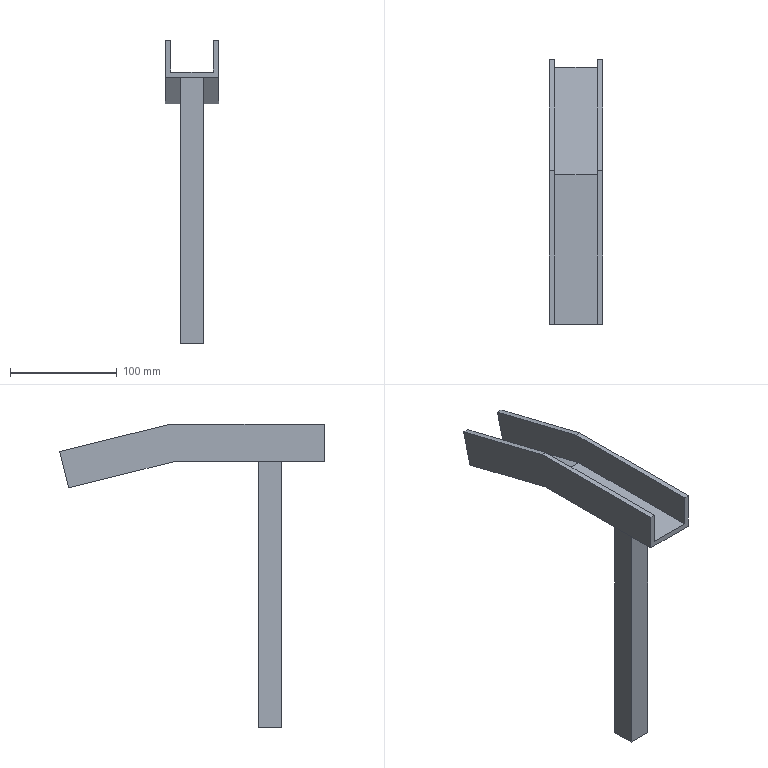Part | NX | features solid 2 | 1 solid | 24 faces | box 50 x 248.417 x 285 mm | volume 175280 mm3 | plane 24
STEP:
#1=CARTESIAN_POINT('',(228.742,734.,15.));
#2=VERTEX_POINT('',#1);
#3=CARTESIAN_POINT('',(228.742,874.61,15.));
#4=VERTEX_POINT('',#3);
#5=CARTESIAN_POINT('',(228.742,829.805,15.));
#6=DIRECTION('',(0.,1.,0.));
#7=VECTOR('',#6,1000.);
#8=LINE('',#5,#7);
#9=EDGE_CURVE('',#2,#4,#8,.T.);
#10=ORIENTED_EDGE('',*,*,#9,.T.);
#11=CARTESIAN_POINT('',(228.742,975.202,-9.923));
#12=VERTEX_POINT('',#11);
#13=CARTESIAN_POINT('',(228.742,924.906,2.538));
#14=DIRECTION('',(0.,0.9707,-0.2405));
#15=VECTOR('',#14,1000.);
#16=LINE('',#13,#15);
#17=EDGE_CURVE('',#4,#12,#16,.T.);
#18=ORIENTED_EDGE('',*,*,#17,.T.);
#19=CARTESIAN_POINT('',(228.742,982.417,19.196));
#20=VERTEX_POINT('',#19);
#21=CARTESIAN_POINT('',(228.742,978.81,4.637));
#22=DIRECTION('',(0.,0.2405,0.9707));
#23=VECTOR('',#22,1000.);
#24=LINE('',#21,#23);
#25=EDGE_CURVE('',#12,#20,#24,.T.);
#26=ORIENTED_EDGE('',*,*,#25,.T.);
#27=CARTESIAN_POINT('',(228.742,878.271,45.));
#28=VERTEX_POINT('',#27);
#29=CARTESIAN_POINT('',(228.742,930.344,32.098));
#30=DIRECTION('',(0.,0.9707,-0.2405));
#31=VECTOR('',#30,1000.);
#32=LINE('',#29,#31);
#33=EDGE_CURVE('',#28,#20,#32,.T.);
#34=ORIENTED_EDGE('',*,*,#33,.F.);
#35=CARTESIAN_POINT('',(228.742,734.,45.));
#36=VERTEX_POINT('',#35);
#37=CARTESIAN_POINT('',(228.742,831.636,45.));
#38=DIRECTION('',(0.,1.,0.));
#39=VECTOR('',#38,1000.);
#40=LINE('',#37,#39);
#41=EDGE_CURVE('',#36,#28,#40,.T.);
#42=ORIENTED_EDGE('',*,*,#41,.F.);
#43=CARTESIAN_POINT('',(228.742,734.,10.));
#44=DIRECTION('',(0.,0.,1.));
#45=VECTOR('',#44,1000.);
#46=LINE('',#43,#45);
#47=EDGE_CURVE('',#2,#36,#46,.T.);
#48=ORIENTED_EDGE('',*,*,#47,.F.);
#49=EDGE_LOOP('',(#10,#18,#26,#34,#42,#48));
#50=FACE_BOUND('',#49,.T.);
#51=CARTESIAN_POINT('',(228.742,831.636,45.));
#52=DIRECTION('',(1.,0.,0.));
#53=DIRECTION('',(0.,0.,1.));
#54=AXIS2_PLACEMENT_3D('',#51,#52,#53);
#55=PLANE('',#54);
#56=ADVANCED_FACE('',(#50),#55,.T.);
#57=CARTESIAN_POINT('',(268.742,734.,15.));
#58=VERTEX_POINT('',#57);
#59=CARTESIAN_POINT('',(268.742,874.61,15.));
#60=VERTEX_POINT('',#59);
#61=CARTESIAN_POINT('',(268.742,829.805,15.));
#62=DIRECTION('',(0.,1.,0.));
#63=VECTOR('',#62,1000.);
#64=LINE('',#61,#63);
#65=EDGE_CURVE('',#58,#60,#64,.T.);
#66=ORIENTED_EDGE('',*,*,#65,.T.);
#67=CARTESIAN_POINT('',(248.742,874.61,15.));
#68=DIRECTION('',(-1.,0.,0.));
#69=VECTOR('',#68,1000.);
#70=LINE('',#67,#69);
#71=EDGE_CURVE('',#60,#4,#70,.T.);
#72=ORIENTED_EDGE('',*,*,#71,.T.);
#73=ORIENTED_EDGE('',*,*,#9,.F.);
#74=CARTESIAN_POINT('',(137.742,734.,15.));
#75=DIRECTION('',(-1.,0.,0.));
#76=VECTOR('',#75,1000.);
#77=LINE('',#74,#76);
#78=EDGE_CURVE('',#58,#2,#77,.T.);
#79=ORIENTED_EDGE('',*,*,#78,.F.);
#80=EDGE_LOOP('',(#66,#72,#73,#79));
#81=FACE_BOUND('',#80,.T.);
#82=CARTESIAN_POINT('',(228.742,829.805,15.));
#83=DIRECTION('',(0.,0.,1.));
#84=DIRECTION('',(0.,1.,0.));
#85=AXIS2_PLACEMENT_3D('',#82,#83,#84);
#86=PLANE('',#85);
#87=ADVANCED_FACE('',(#81),#86,.T.);
#88=CARTESIAN_POINT('',(268.742,734.,45.));
#89=VERTEX_POINT('',#88);
#90=CARTESIAN_POINT('',(268.742,878.271,45.));
#91=VERTEX_POINT('',#90);
#92=CARTESIAN_POINT('',(268.742,831.636,45.));
#93=DIRECTION('',(0.,1.,0.));
#94=VECTOR('',#93,1000.);
#95=LINE('',#92,#94);
#96=EDGE_CURVE('',#89,#91,#95,.T.);
#97=ORIENTED_EDGE('',*,*,#96,.T.);
#98=CARTESIAN_POINT('',(268.742,982.417,19.196));
#99=VERTEX_POINT('',#98);
#100=CARTESIAN_POINT('',(268.742,930.344,32.098));
#101=DIRECTION('',(0.,0.9707,-0.2405));
#102=VECTOR('',#101,1000.);
#103=LINE('',#100,#102);
#104=EDGE_CURVE('',#91,#99,#103,.T.);
#105=ORIENTED_EDGE('',*,*,#104,.T.);
#106=CARTESIAN_POINT('',(268.742,975.202,-9.923));
#107=VERTEX_POINT('',#106);
#108=CARTESIAN_POINT('',(268.742,978.81,4.637));
#109=DIRECTION('',(0.,-0.2405,-0.9707));
#110=VECTOR('',#109,1000.);
#111=LINE('',#108,#110);
#112=EDGE_CURVE('',#99,#107,#111,.T.);
#113=ORIENTED_EDGE('',*,*,#112,.T.);
#114=CARTESIAN_POINT('',(268.742,924.906,2.538));
#115=DIRECTION('',(0.,0.9707,-0.2405));
#116=VECTOR('',#115,1000.);
#117=LINE('',#114,#116);
#118=EDGE_CURVE('',#60,#107,#117,.T.);
#119=ORIENTED_EDGE('',*,*,#118,.F.);
#120=ORIENTED_EDGE('',*,*,#65,.F.);
#121=CARTESIAN_POINT('',(268.742,734.,10.));
#122=DIRECTION('',(0.,0.,-1.));
#123=VECTOR('',#122,1000.);
#124=LINE('',#121,#123);
#125=EDGE_CURVE('',#89,#58,#124,.T.);
#126=ORIENTED_EDGE('',*,*,#125,.F.);
#127=EDGE_LOOP('',(#97,#105,#113,#119,#120,#126));
#128=FACE_BOUND('',#127,.T.);
#129=CARTESIAN_POINT('',(268.742,831.636,45.));
#130=DIRECTION('',(-1.,0.,0.));
#131=DIRECTION('',(0.,0.,-1.));
#132=AXIS2_PLACEMENT_3D('',#129,#130,#131);
#133=PLANE('',#132);
#134=ADVANCED_FACE('',(#128),#133,.T.);
#135=CARTESIAN_POINT('',(273.742,734.,45.));
#136=VERTEX_POINT('',#135);
#137=CARTESIAN_POINT('',(273.742,878.271,45.));
#138=VERTEX_POINT('',#137);
#139=CARTESIAN_POINT('',(273.742,831.636,45.));
#140=DIRECTION('',(0.,1.,0.));
#141=VECTOR('',#140,1000.);
#142=LINE('',#139,#141);
#143=EDGE_CURVE('',#136,#138,#142,.T.);
#144=ORIENTED_EDGE('',*,*,#143,.T.);
#145=CARTESIAN_POINT('',(271.242,878.271,45.));
#146=DIRECTION('',(-1.,0.,0.));
#147=VECTOR('',#146,1000.);
#148=LINE('',#145,#147);
#149=EDGE_CURVE('',#138,#91,#148,.T.);
#150=ORIENTED_EDGE('',*,*,#149,.T.);
#151=ORIENTED_EDGE('',*,*,#96,.F.);
#152=CARTESIAN_POINT('',(137.742,734.,45.));
#153=DIRECTION('',(-1.,0.,0.));
#154=VECTOR('',#153,1000.);
#155=LINE('',#152,#154);
#156=EDGE_CURVE('',#136,#89,#155,.T.);
#157=ORIENTED_EDGE('',*,*,#156,.F.);
#158=EDGE_LOOP('',(#144,#150,#151,#157));
#159=FACE_BOUND('',#158,.T.);
#160=CARTESIAN_POINT('',(268.742,831.636,45.));
#161=DIRECTION('',(0.,0.,1.));
#162=DIRECTION('',(0.,1.,0.));
#163=AXIS2_PLACEMENT_3D('',#160,#161,#162);
#164=PLANE('',#163);
#165=ADVANCED_FACE('',(#159),#164,.T.);
#166=CARTESIAN_POINT('',(273.742,734.,10.));
#167=VERTEX_POINT('',#166);
#168=CARTESIAN_POINT('',(273.742,874.,10.));
#169=VERTEX_POINT('',#168);
#170=CARTESIAN_POINT('',(273.742,829.5,10.));
#171=DIRECTION('',(0.,1.,0.));
#172=VECTOR('',#171,1000.);
#173=LINE('',#170,#172);
#174=EDGE_CURVE('',#167,#169,#173,.T.);
#175=ORIENTED_EDGE('',*,*,#174,.T.);
#176=CARTESIAN_POINT('',(273.742,974.,-14.776));
#177=VERTEX_POINT('',#176);
#178=CARTESIAN_POINT('',(273.742,924.,-2.388));
#179=DIRECTION('',(0.,0.9707,-0.2405));
#180=VECTOR('',#179,1000.);
#181=LINE('',#178,#180);
#182=EDGE_CURVE('',#169,#177,#181,.T.);
#183=ORIENTED_EDGE('',*,*,#182,.T.);
#184=CARTESIAN_POINT('',(273.742,982.417,19.196));
#185=VERTEX_POINT('',#184);
#186=CARTESIAN_POINT('',(273.742,978.209,2.21));
#187=DIRECTION('',(0.,0.2405,0.9707));
#188=VECTOR('',#187,1000.);
#189=LINE('',#186,#188);
#190=EDGE_CURVE('',#177,#185,#189,.T.);
#191=ORIENTED_EDGE('',*,*,#190,.T.);
#192=CARTESIAN_POINT('',(273.742,930.344,32.098));
#193=DIRECTION('',(0.,0.9707,-0.2405));
#194=VECTOR('',#193,1000.);
#195=LINE('',#192,#194);
#196=EDGE_CURVE('',#138,#185,#195,.T.);
#197=ORIENTED_EDGE('',*,*,#196,.F.);
#198=ORIENTED_EDGE('',*,*,#143,.F.);
#199=CARTESIAN_POINT('',(273.742,734.,10.));
#200=DIRECTION('',(0.,0.,1.));
#201=VECTOR('',#200,1000.);
#202=LINE('',#199,#201);
#203=EDGE_CURVE('',#167,#136,#202,.T.);
#204=ORIENTED_EDGE('',*,*,#203,.F.);
#205=EDGE_LOOP('',(#175,#183,#191,#197,#198,#204));
#206=FACE_BOUND('',#205,.T.);
#207=CARTESIAN_POINT('',(273.742,831.636,45.));
#208=DIRECTION('',(1.,0.,0.));
#209=DIRECTION('',(0.,0.,1.));
#210=AXIS2_PLACEMENT_3D('',#207,#208,#209);
#211=PLANE('',#210);
#212=ADVANCED_FACE('',(#206),#211,.T.);
#213=CARTESIAN_POINT('',(237.742,774.,10.));
#214=VERTEX_POINT('',#213);
#215=CARTESIAN_POINT('',(259.742,774.,10.));
#216=VERTEX_POINT('',#215);
#217=CARTESIAN_POINT('',(237.742,774.,10.));
#218=DIRECTION('',(1.,0.,0.));
#219=VECTOR('',#218,1000.);
#220=LINE('',#217,#219);
#221=EDGE_CURVE('',#214,#216,#220,.T.);
#222=ORIENTED_EDGE('',*,*,#221,.T.);
#223=CARTESIAN_POINT('',(259.742,796.,10.));
#224=VERTEX_POINT('',#223);
#225=CARTESIAN_POINT('',(259.742,774.,10.));
#226=DIRECTION('',(0.,1.,0.));
#227=VECTOR('',#226,1000.);
#228=LINE('',#225,#227);
#229=EDGE_CURVE('',#216,#224,#228,.T.);
#230=ORIENTED_EDGE('',*,*,#229,.T.);
#231=CARTESIAN_POINT('',(237.742,796.,10.));
#232=VERTEX_POINT('',#231);
#233=CARTESIAN_POINT('',(259.742,796.,10.));
#234=DIRECTION('',(-1.,0.,0.));
#235=VECTOR('',#234,1000.);
#236=LINE('',#233,#235);
#237=EDGE_CURVE('',#224,#232,#236,.T.);
#238=ORIENTED_EDGE('',*,*,#237,.T.);
#239=CARTESIAN_POINT('',(237.742,796.,10.));
#240=DIRECTION('',(0.,-1.,0.));
#241=VECTOR('',#240,1000.);
#242=LINE('',#239,#241);
#243=EDGE_CURVE('',#232,#214,#242,.T.);
#244=ORIENTED_EDGE('',*,*,#243,.T.);
#245=EDGE_LOOP('',(#222,#230,#238,#244));
#246=FACE_BOUND('',#245,.T.);
#247=CARTESIAN_POINT('',(223.742,734.,10.));
#248=VERTEX_POINT('',#247);
#249=CARTESIAN_POINT('',(223.742,874.,10.));
#250=VERTEX_POINT('',#249);
#251=CARTESIAN_POINT('',(223.742,829.5,10.));
#252=DIRECTION('',(0.,1.,0.));
#253=VECTOR('',#252,1000.);
#254=LINE('',#251,#253);
#255=EDGE_CURVE('',#248,#250,#254,.T.);
#256=ORIENTED_EDGE('',*,*,#255,.T.);
#257=CARTESIAN_POINT('',(248.742,874.,10.));
#258=DIRECTION('',(1.,0.,0.));
#259=VECTOR('',#258,1000.);
#260=LINE('',#257,#259);
#261=EDGE_CURVE('',#250,#169,#260,.T.);
#262=ORIENTED_EDGE('',*,*,#261,.T.);
#263=ORIENTED_EDGE('',*,*,#174,.F.);
#264=CARTESIAN_POINT('',(137.742,734.,10.));
#265=DIRECTION('',(1.,0.,0.));
#266=VECTOR('',#265,1000.);
#267=LINE('',#264,#266);
#268=EDGE_CURVE('',#248,#167,#267,.T.);
#269=ORIENTED_EDGE('',*,*,#268,.F.);
#270=EDGE_LOOP('',(#256,#262,#263,#269));
#271=FACE_BOUND('',#270,.T.);
#272=CARTESIAN_POINT('',(273.742,829.5,10.));
#273=DIRECTION('',(0.,0.,-1.));
#274=DIRECTION('',(0.,-1.,0.));
#275=AXIS2_PLACEMENT_3D('',#272,#273,#274);
#276=PLANE('',#275);
#277=ADVANCED_FACE('',(#246,#271),#276,.T.);
#278=ORIENTED_EDGE('',*,*,#41,.T.);
#279=CARTESIAN_POINT('',(223.742,878.271,45.));
#280=VERTEX_POINT('',#279);
#281=CARTESIAN_POINT('',(226.242,878.271,45.));
#282=DIRECTION('',(-1.,0.,0.));
#283=VECTOR('',#282,1000.);
#284=LINE('',#281,#283);
#285=EDGE_CURVE('',#28,#280,#284,.T.);
#286=ORIENTED_EDGE('',*,*,#285,.T.);
#287=CARTESIAN_POINT('',(223.742,734.,45.));
#288=VERTEX_POINT('',#287);
#289=CARTESIAN_POINT('',(223.742,831.636,45.));
#290=DIRECTION('',(0.,1.,0.));
#291=VECTOR('',#290,1000.);
#292=LINE('',#289,#291);
#293=EDGE_CURVE('',#288,#280,#292,.T.);
#294=ORIENTED_EDGE('',*,*,#293,.F.);
#295=CARTESIAN_POINT('',(137.742,734.,45.));
#296=DIRECTION('',(-1.,0.,0.));
#297=VECTOR('',#296,1000.);
#298=LINE('',#295,#297);
#299=EDGE_CURVE('',#36,#288,#298,.T.);
#300=ORIENTED_EDGE('',*,*,#299,.F.);
#301=EDGE_LOOP('',(#278,#286,#294,#300));
#302=FACE_BOUND('',#301,.T.);
#303=CARTESIAN_POINT('',(223.742,831.636,45.));
#304=DIRECTION('',(0.,0.,1.));
#305=DIRECTION('',(0.,1.,0.));
#306=AXIS2_PLACEMENT_3D('',#303,#304,#305);
#307=PLANE('',#306);
#308=ADVANCED_FACE('',(#302),#307,.T.);
#309=ORIENTED_EDGE('',*,*,#293,.T.);
#310=CARTESIAN_POINT('',(223.742,982.417,19.196));
#311=VERTEX_POINT('',#310);
#312=CARTESIAN_POINT('',(223.742,930.344,32.098));
#313=DIRECTION('',(0.,0.9707,-0.2405));
#314=VECTOR('',#313,1000.);
#315=LINE('',#312,#314);
#316=EDGE_CURVE('',#280,#311,#315,.T.);
#317=ORIENTED_EDGE('',*,*,#316,.T.);
#318=CARTESIAN_POINT('',(223.742,974.,-14.776));
#319=VERTEX_POINT('',#318);
#320=CARTESIAN_POINT('',(223.742,978.209,2.21));
#321=DIRECTION('',(0.,-0.2405,-0.9707));
#322=VECTOR('',#321,1000.);
#323=LINE('',#320,#322);
#324=EDGE_CURVE('',#311,#319,#323,.T.);
#325=ORIENTED_EDGE('',*,*,#324,.T.);
#326=CARTESIAN_POINT('',(223.742,924.,-2.388));
#327=DIRECTION('',(0.,0.9707,-0.2405));
#328=VECTOR('',#327,1000.);
#329=LINE('',#326,#328);
#330=EDGE_CURVE('',#250,#319,#329,.T.);
#331=ORIENTED_EDGE('',*,*,#330,.F.);
#332=ORIENTED_EDGE('',*,*,#255,.F.);
#333=CARTESIAN_POINT('',(223.742,734.,10.));
#334=DIRECTION('',(0.,0.,-1.));
#335=VECTOR('',#334,1000.);
#336=LINE('',#333,#335);
#337=EDGE_CURVE('',#288,#248,#336,.T.);
#338=ORIENTED_EDGE('',*,*,#337,.F.);
#339=EDGE_LOOP('',(#309,#317,#325,#331,#332,#338));
#340=FACE_BOUND('',#339,.T.);
#341=CARTESIAN_POINT('',(223.742,831.636,45.));
#342=DIRECTION('',(-1.,0.,0.));
#343=DIRECTION('',(0.,0.,-1.));
#344=AXIS2_PLACEMENT_3D('',#341,#342,#343);
#345=PLANE('',#344);
#346=ADVANCED_FACE('',(#340),#345,.T.);
#347=CARTESIAN_POINT('',(237.742,796.,-240.));
#348=VERTEX_POINT('',#347);
#349=CARTESIAN_POINT('',(237.742,774.,-240.));
#350=VERTEX_POINT('',#349);
#351=CARTESIAN_POINT('',(237.742,796.,-240.));
#352=DIRECTION('',(0.,-1.,0.));
#353=VECTOR('',#352,1000.);
#354=LINE('',#351,#353);
#355=EDGE_CURVE('',#348,#350,#354,.T.);
#356=ORIENTED_EDGE('',*,*,#355,.T.);
#357=CARTESIAN_POINT('',(237.742,774.,10.));
#358=DIRECTION('',(0.,0.,-1.));
#359=VECTOR('',#358,1000.);
#360=LINE('',#357,#359);
#361=EDGE_CURVE('',#214,#350,#360,.T.);
#362=ORIENTED_EDGE('',*,*,#361,.F.);
#363=ORIENTED_EDGE('',*,*,#243,.F.);
#364=CARTESIAN_POINT('',(237.742,796.,10.));
#365=DIRECTION('',(0.,0.,-1.));
#366=VECTOR('',#365,1000.);
#367=LINE('',#364,#366);
#368=EDGE_CURVE('',#232,#348,#367,.T.);
#369=ORIENTED_EDGE('',*,*,#368,.T.);
#370=EDGE_LOOP('',(#356,#362,#363,#369));
#371=FACE_BOUND('',#370,.T.);
#372=CARTESIAN_POINT('',(237.742,796.,10.));
#373=DIRECTION('',(-1.,0.,0.));
#374=DIRECTION('',(0.,1.,0.));
#375=AXIS2_PLACEMENT_3D('',#372,#373,#374);
#376=PLANE('',#375);
#377=ADVANCED_FACE('',(#371),#376,.T.);
#378=CARTESIAN_POINT('',(259.742,774.,-240.));
#379=VERTEX_POINT('',#378);
#380=CARTESIAN_POINT('',(237.742,774.,-240.));
#381=DIRECTION('',(1.,0.,0.));
#382=VECTOR('',#381,1000.);
#383=LINE('',#380,#382);
#384=EDGE_CURVE('',#350,#379,#383,.T.);
#385=ORIENTED_EDGE('',*,*,#384,.T.);
#386=CARTESIAN_POINT('',(259.742,774.,10.));
#387=DIRECTION('',(0.,0.,-1.));
#388=VECTOR('',#387,1000.);
#389=LINE('',#386,#388);
#390=EDGE_CURVE('',#216,#379,#389,.T.);
#391=ORIENTED_EDGE('',*,*,#390,.F.);
#392=ORIENTED_EDGE('',*,*,#221,.F.);
#393=ORIENTED_EDGE('',*,*,#361,.T.);
#394=EDGE_LOOP('',(#385,#391,#392,#393));
#395=FACE_BOUND('',#394,.T.);
#396=CARTESIAN_POINT('',(237.742,774.,10.));
#397=DIRECTION('',(0.,-1.,0.));
#398=DIRECTION('',(0.,0.,1.));
#399=AXIS2_PLACEMENT_3D('',#396,#397,#398);
#400=PLANE('',#399);
#401=ADVANCED_FACE('',(#395),#400,.T.);
#402=CARTESIAN_POINT('',(259.742,796.,-240.));
#403=VERTEX_POINT('',#402);
#404=CARTESIAN_POINT('',(259.742,774.,-240.));
#405=DIRECTION('',(0.,1.,0.));
#406=VECTOR('',#405,1000.);
#407=LINE('',#404,#406);
#408=EDGE_CURVE('',#379,#403,#407,.T.);
#409=ORIENTED_EDGE('',*,*,#408,.T.);
#410=CARTESIAN_POINT('',(259.742,796.,10.));
#411=DIRECTION('',(0.,0.,-1.));
#412=VECTOR('',#411,1000.);
#413=LINE('',#410,#412);
#414=EDGE_CURVE('',#224,#403,#413,.T.);
#415=ORIENTED_EDGE('',*,*,#414,.F.);
#416=ORIENTED_EDGE('',*,*,#229,.F.);
#417=ORIENTED_EDGE('',*,*,#390,.T.);
#418=EDGE_LOOP('',(#409,#415,#416,#417));
#419=FACE_BOUND('',#418,.T.);
#420=CARTESIAN_POINT('',(259.742,774.,10.));
#421=DIRECTION('',(1.,0.,0.));
#422=DIRECTION('',(0.,0.,1.));
#423=AXIS2_PLACEMENT_3D('',#420,#421,#422);
#424=PLANE('',#423);
#425=ADVANCED_FACE('',(#419),#424,.T.);
#426=CARTESIAN_POINT('',(239.742,776.,-240.));
#427=VERTEX_POINT('',#426);
#428=CARTESIAN_POINT('',(257.742,776.,-240.));
#429=VERTEX_POINT('',#428);
#430=CARTESIAN_POINT('',(239.742,776.,-240.));
#431=DIRECTION('',(1.,0.,0.));
#432=VECTOR('',#431,1000.);
#433=LINE('',#430,#432);
#434=EDGE_CURVE('',#427,#429,#433,.T.);
#435=ORIENTED_EDGE('',*,*,#434,.F.);
#436=CARTESIAN_POINT('',(239.742,776.,10.));
#437=VERTEX_POINT('',#436);
#438=CARTESIAN_POINT('',(239.742,776.,10.));
#439=DIRECTION('',(0.,0.,-1.));
#440=VECTOR('',#439,1000.);
#441=LINE('',#438,#440);
#442=EDGE_CURVE('',#437,#427,#441,.T.);
#443=ORIENTED_EDGE('',*,*,#442,.F.);
#444=CARTESIAN_POINT('',(257.742,776.,10.));
#445=VERTEX_POINT('',#444);
#446=CARTESIAN_POINT('',(239.742,776.,10.));
#447=DIRECTION('',(1.,0.,0.));
#448=VECTOR('',#447,1000.);
#449=LINE('',#446,#448);
#450=EDGE_CURVE('',#437,#445,#449,.T.);
#451=ORIENTED_EDGE('',*,*,#450,.T.);
#452=CARTESIAN_POINT('',(257.742,776.,10.));
#453=DIRECTION('',(0.,0.,-1.));
#454=VECTOR('',#453,1000.);
#455=LINE('',#452,#454);
#456=EDGE_CURVE('',#445,#429,#455,.T.);
#457=ORIENTED_EDGE('',*,*,#456,.T.);
#458=EDGE_LOOP('',(#435,#443,#451,#457));
#459=FACE_BOUND('',#458,.T.);
#460=CARTESIAN_POINT('',(239.742,776.,10.));
#461=DIRECTION('',(0.,-1.,0.));
#462=DIRECTION('',(-1.,0.,0.));
#463=AXIS2_PLACEMENT_3D('',#460,#461,#462);
#464=PLANE('',#463);
#465=ADVANCED_FACE('',(#459),#464,.F.);
#466=CARTESIAN_POINT('',(239.742,794.,-240.));
#467=VERTEX_POINT('',#466);
#468=CARTESIAN_POINT('',(239.742,794.,-240.));
#469=DIRECTION('',(0.,-1.,0.));
#470=VECTOR('',#469,1000.);
#471=LINE('',#468,#470);
#472=EDGE_CURVE('',#467,#427,#471,.T.);
#473=ORIENTED_EDGE('',*,*,#472,.F.);
#474=CARTESIAN_POINT('',(239.742,794.,10.));
#475=VERTEX_POINT('',#474);
#476=CARTESIAN_POINT('',(239.742,794.,10.));
#477=DIRECTION('',(0.,0.,-1.));
#478=VECTOR('',#477,1000.);
#479=LINE('',#476,#478);
#480=EDGE_CURVE('',#475,#467,#479,.T.);
#481=ORIENTED_EDGE('',*,*,#480,.F.);
#482=CARTESIAN_POINT('',(239.742,794.,10.));
#483=DIRECTION('',(0.,-1.,0.));
#484=VECTOR('',#483,1000.);
#485=LINE('',#482,#484);
#486=EDGE_CURVE('',#475,#437,#485,.T.);
#487=ORIENTED_EDGE('',*,*,#486,.T.);
#488=ORIENTED_EDGE('',*,*,#442,.T.);
#489=EDGE_LOOP('',(#473,#481,#487,#488));
#490=FACE_BOUND('',#489,.T.);
#491=CARTESIAN_POINT('',(239.742,794.,10.));
#492=DIRECTION('',(-1.,0.,0.));
#493=DIRECTION('',(0.,1.,0.));
#494=AXIS2_PLACEMENT_3D('',#491,#492,#493);
#495=PLANE('',#494);
#496=ADVANCED_FACE('',(#490),#495,.F.);
#497=CARTESIAN_POINT('',(257.742,794.,-240.));
#498=VERTEX_POINT('',#497);
#499=CARTESIAN_POINT('',(257.742,794.,-240.));
#500=DIRECTION('',(-1.,0.,0.));
#501=VECTOR('',#500,1000.);
#502=LINE('',#499,#501);
#503=EDGE_CURVE('',#498,#467,#502,.T.);
#504=ORIENTED_EDGE('',*,*,#503,.F.);
#505=CARTESIAN_POINT('',(257.742,794.,10.));
#506=VERTEX_POINT('',#505);
#507=CARTESIAN_POINT('',(257.742,794.,10.));
#508=DIRECTION('',(0.,0.,-1.));
#509=VECTOR('',#508,1000.);
#510=LINE('',#507,#509);
#511=EDGE_CURVE('',#506,#498,#510,.T.);
#512=ORIENTED_EDGE('',*,*,#511,.F.);
#513=CARTESIAN_POINT('',(257.742,794.,10.));
#514=DIRECTION('',(-1.,0.,0.));
#515=VECTOR('',#514,1000.);
#516=LINE('',#513,#515);
#517=EDGE_CURVE('',#506,#475,#516,.T.);
#518=ORIENTED_EDGE('',*,*,#517,.T.);
#519=ORIENTED_EDGE('',*,*,#480,.T.);
#520=EDGE_LOOP('',(#504,#512,#518,#519));
#521=FACE_BOUND('',#520,.T.);
#522=CARTESIAN_POINT('',(257.742,794.,10.));
#523=DIRECTION('',(0.,1.,0.));
#524=DIRECTION('',(1.,0.,0.));
#525=AXIS2_PLACEMENT_3D('',#522,#523,#524);
#526=PLANE('',#525);
#527=ADVANCED_FACE('',(#521),#526,.F.);
#528=CARTESIAN_POINT('',(257.742,776.,-240.));
#529=DIRECTION('',(0.,1.,0.));
#530=VECTOR('',#529,1000.);
#531=LINE('',#528,#530);
#532=EDGE_CURVE('',#429,#498,#531,.T.);
#533=ORIENTED_EDGE('',*,*,#532,.F.);
#534=ORIENTED_EDGE('',*,*,#456,.F.);
#535=CARTESIAN_POINT('',(257.742,776.,10.));
#536=DIRECTION('',(0.,1.,0.));
#537=VECTOR('',#536,1000.);
#538=LINE('',#535,#537);
#539=EDGE_CURVE('',#445,#506,#538,.T.);
#540=ORIENTED_EDGE('',*,*,#539,.T.);
#541=ORIENTED_EDGE('',*,*,#511,.T.);
#542=EDGE_LOOP('',(#533,#534,#540,#541));
#543=FACE_BOUND('',#542,.T.);
#544=CARTESIAN_POINT('',(257.742,776.,10.));
#545=DIRECTION('',(1.,0.,0.));
#546=DIRECTION('',(0.,0.,1.));
#547=AXIS2_PLACEMENT_3D('',#544,#545,#546);
#548=PLANE('',#547);
#549=ADVANCED_FACE('',(#543),#548,.F.);
#550=CARTESIAN_POINT('',(259.742,796.,-240.));
#551=DIRECTION('',(-1.,0.,0.));
#552=VECTOR('',#551,1000.);
#553=LINE('',#550,#552);
#554=EDGE_CURVE('',#403,#348,#553,.T.);
#555=ORIENTED_EDGE('',*,*,#554,.T.);
#556=ORIENTED_EDGE('',*,*,#368,.F.);
#557=ORIENTED_EDGE('',*,*,#237,.F.);
#558=ORIENTED_EDGE('',*,*,#414,.T.);
#559=EDGE_LOOP('',(#555,#556,#557,#558));
#560=FACE_BOUND('',#559,.T.);
#561=CARTESIAN_POINT('',(259.742,796.,10.));
#562=DIRECTION('',(0.,1.,0.));
#563=DIRECTION('',(0.,0.,-1.));
#564=AXIS2_PLACEMENT_3D('',#561,#562,#563);
#565=PLANE('',#564);
#566=ADVANCED_FACE('',(#560),#565,.T.);
#567=ORIENTED_EDGE('',*,*,#434,.T.);
#568=ORIENTED_EDGE('',*,*,#532,.T.);
#569=ORIENTED_EDGE('',*,*,#503,.T.);
#570=ORIENTED_EDGE('',*,*,#472,.T.);
#571=EDGE_LOOP('',(#567,#568,#569,#570));
#572=FACE_BOUND('',#571,.T.);
#573=ORIENTED_EDGE('',*,*,#355,.F.);
#574=ORIENTED_EDGE('',*,*,#554,.F.);
#575=ORIENTED_EDGE('',*,*,#408,.F.);
#576=ORIENTED_EDGE('',*,*,#384,.F.);
#577=EDGE_LOOP('',(#573,#574,#575,#576));
#578=FACE_BOUND('',#577,.T.);
#579=CARTESIAN_POINT('',(237.742,774.,-240.));
#580=DIRECTION('',(0.,0.,-1.));
#581=DIRECTION('',(0.,-1.,0.));
#582=AXIS2_PLACEMENT_3D('',#579,#580,#581);
#583=PLANE('',#582);
#584=ADVANCED_FACE('',(#572,#578),#583,.T.);
#585=ORIENTED_EDGE('',*,*,#25,.F.);
#586=CARTESIAN_POINT('',(248.742,975.202,-9.923));
#587=DIRECTION('',(-1.,0.,0.));
#588=VECTOR('',#587,1000.);
#589=LINE('',#586,#588);
#590=EDGE_CURVE('',#107,#12,#589,.T.);
#591=ORIENTED_EDGE('',*,*,#590,.F.);
#592=ORIENTED_EDGE('',*,*,#112,.F.);
#593=CARTESIAN_POINT('',(271.242,982.417,19.196));
#594=DIRECTION('',(-1.,0.,0.));
#595=VECTOR('',#594,1000.);
#596=LINE('',#593,#595);
#597=EDGE_CURVE('',#185,#99,#596,.T.);
#598=ORIENTED_EDGE('',*,*,#597,.F.);
#599=ORIENTED_EDGE('',*,*,#190,.F.);
#600=CARTESIAN_POINT('',(248.742,974.,-14.776));
#601=DIRECTION('',(1.,0.,0.));
#602=VECTOR('',#601,1000.);
#603=LINE('',#600,#602);
#604=EDGE_CURVE('',#319,#177,#603,.T.);
#605=ORIENTED_EDGE('',*,*,#604,.F.);
#606=ORIENTED_EDGE('',*,*,#324,.F.);
#607=CARTESIAN_POINT('',(226.242,982.417,19.196));
#608=DIRECTION('',(-1.,0.,0.));
#609=VECTOR('',#608,1000.);
#610=LINE('',#607,#609);
#611=EDGE_CURVE('',#20,#311,#610,.T.);
#612=ORIENTED_EDGE('',*,*,#611,.F.);
#613=EDGE_LOOP('',(#585,#591,#592,#598,#599,#605,#606,#612));
#614=FACE_BOUND('',#613,.T.);
#615=CARTESIAN_POINT('',(248.742,974.,-14.776));
#616=DIRECTION('',(0.,0.9707,-0.2405));
#617=DIRECTION('',(0.,-0.2405,-0.9707));
#618=AXIS2_PLACEMENT_3D('',#615,#616,#617);
#619=PLANE('',#618);
#620=ADVANCED_FACE('',(#614),#619,.T.);
#621=ORIENTED_EDGE('',*,*,#33,.T.);
#622=ORIENTED_EDGE('',*,*,#611,.T.);
#623=ORIENTED_EDGE('',*,*,#316,.F.);
#624=ORIENTED_EDGE('',*,*,#285,.F.);
#625=EDGE_LOOP('',(#621,#622,#623,#624));
#626=FACE_BOUND('',#625,.T.);
#627=CARTESIAN_POINT('',(223.742,930.344,32.098));
#628=DIRECTION('',(0.,0.2405,0.9707));
#629=DIRECTION('',(0.,0.9707,-0.2405));
#630=AXIS2_PLACEMENT_3D('',#627,#628,#629);
#631=PLANE('',#630);
#632=ADVANCED_FACE('',(#626),#631,.T.);
#633=ORIENTED_EDGE('',*,*,#118,.T.);
#634=ORIENTED_EDGE('',*,*,#590,.T.);
#635=ORIENTED_EDGE('',*,*,#17,.F.);
#636=ORIENTED_EDGE('',*,*,#71,.F.);
#637=EDGE_LOOP('',(#633,#634,#635,#636));
#638=FACE_BOUND('',#637,.T.);
#639=CARTESIAN_POINT('',(228.742,924.906,2.538));
#640=DIRECTION('',(0.,0.2405,0.9707));
#641=DIRECTION('',(0.,0.9707,-0.2405));
#642=AXIS2_PLACEMENT_3D('',#639,#640,#641);
#643=PLANE('',#642);
#644=ADVANCED_FACE('',(#638),#643,.T.);
#645=ORIENTED_EDGE('',*,*,#196,.T.);
#646=ORIENTED_EDGE('',*,*,#597,.T.);
#647=ORIENTED_EDGE('',*,*,#104,.F.);
#648=ORIENTED_EDGE('',*,*,#149,.F.);
#649=EDGE_LOOP('',(#645,#646,#647,#648));
#650=FACE_BOUND('',#649,.T.);
#651=CARTESIAN_POINT('',(268.742,930.344,32.098));
#652=DIRECTION('',(0.,0.2405,0.9707));
#653=DIRECTION('',(0.,0.9707,-0.2405));
#654=AXIS2_PLACEMENT_3D('',#651,#652,#653);
#655=PLANE('',#654);
#656=ADVANCED_FACE('',(#650),#655,.T.);
#657=ORIENTED_EDGE('',*,*,#330,.T.);
#658=ORIENTED_EDGE('',*,*,#604,.T.);
#659=ORIENTED_EDGE('',*,*,#182,.F.);
#660=ORIENTED_EDGE('',*,*,#261,.F.);
#661=EDGE_LOOP('',(#657,#658,#659,#660));
#662=FACE_BOUND('',#661,.T.);
#663=CARTESIAN_POINT('',(273.742,924.,-2.388));
#664=DIRECTION('',(0.,-0.2405,-0.9707));
#665=DIRECTION('',(0.,-0.9707,0.2405));
#666=AXIS2_PLACEMENT_3D('',#663,#664,#665);
#667=PLANE('',#666);
#668=ADVANCED_FACE('',(#662),#667,.T.);
#669=ORIENTED_EDGE('',*,*,#450,.F.);
#670=ORIENTED_EDGE('',*,*,#486,.F.);
#671=ORIENTED_EDGE('',*,*,#517,.F.);
#672=ORIENTED_EDGE('',*,*,#539,.F.);
#673=EDGE_LOOP('',(#669,#670,#671,#672));
#674=FACE_BOUND('',#673,.T.);
#675=CARTESIAN_POINT('',(273.742,829.5,10.));
#676=DIRECTION('',(0.,0.,-1.));
#677=DIRECTION('',(0.,-1.,0.));
#678=AXIS2_PLACEMENT_3D('',#675,#676,#677);
#679=PLANE('',#678);
#680=ADVANCED_FACE('',(#674),#679,.T.);
#681=ORIENTED_EDGE('',*,*,#47,.T.);
#682=ORIENTED_EDGE('',*,*,#299,.T.);
#683=ORIENTED_EDGE('',*,*,#337,.T.);
#684=ORIENTED_EDGE('',*,*,#268,.T.);
#685=ORIENTED_EDGE('',*,*,#203,.T.);
#686=ORIENTED_EDGE('',*,*,#156,.T.);
#687=ORIENTED_EDGE('',*,*,#125,.T.);
#688=ORIENTED_EDGE('',*,*,#78,.T.);
#689=EDGE_LOOP('',(#681,#682,#683,#684,#685,#686,#687,#688));
#690=FACE_BOUND('',#689,.T.);
#691=CARTESIAN_POINT('',(137.742,734.,10.));
#692=DIRECTION('',(0.,-1.,0.));
#693=DIRECTION('',(0.,0.,1.));
#694=AXIS2_PLACEMENT_3D('',#691,#692,#693);
#695=PLANE('',#694);
#696=ADVANCED_FACE('',(#690),#695,.T.);
#697=CLOSED_SHELL('',(#56,#87,#134,#165,#212,#277,#308,#346,#377,#401,#425,#465,#496,#527,#549,#566,#584,#620,#632,#644,#656,#668,#680,#696));
#698=MANIFOLD_SOLID_BREP('',#697);
#699=(LENGTH_UNIT()NAMED_UNIT(*)SI_UNIT(.MILLI.,.METRE.));
#700=UNCERTAINTY_MEASURE_WITH_UNIT(LENGTH_MEASURE(0.00001),#699,'','');
#701=(NAMED_UNIT(*)PLANE_ANGLE_UNIT()SI_UNIT($,.RADIAN.));
#702=(NAMED_UNIT(*)SI_UNIT($,.STERADIAN.)SOLID_ANGLE_UNIT());
#703=(GEOMETRIC_REPRESENTATION_CONTEXT(3)GLOBAL_UNCERTAINTY_ASSIGNED_CONTEXT((#700))GLOBAL_UNIT_ASSIGNED_CONTEXT((#699,#701,#702))REPRESENTATION_CONTEXT('',''));
#704=ADVANCED_BREP_SHAPE_REPRESENTATION('',(#698),#703);